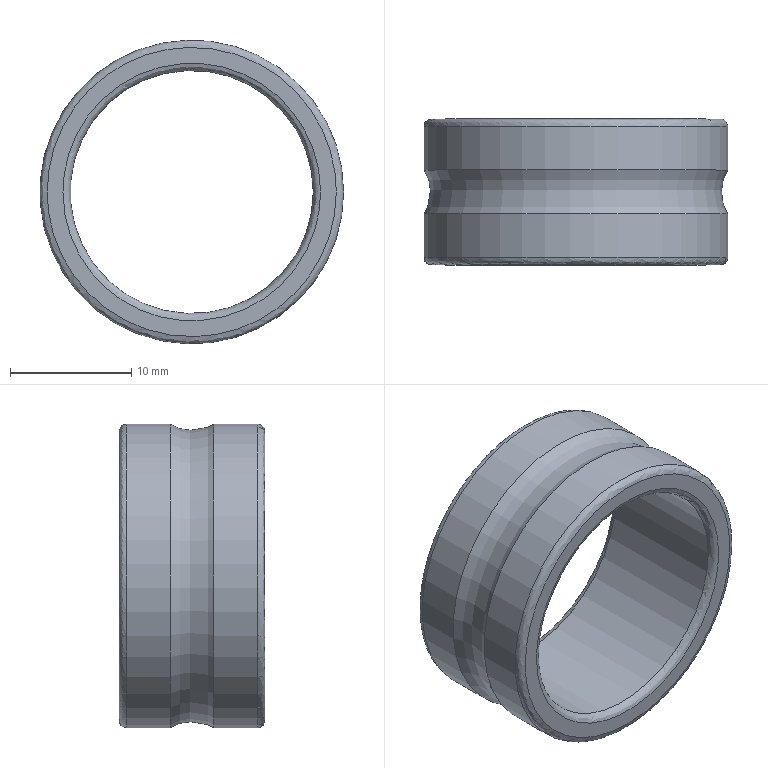Part | STEP file | BF-20_id1366_x_t | 1 solid | 10 faces | box 25 x 12 x 25 mm | volume 2005 mm3 | other 5 | cylinder 3 | plane 2 | commonest cylinder face diameters 25 x2 20 x1
STEP:
#1=CARTESIAN_POINT('',(0.,0.,0.));
#2=DIRECTION('',(0.,0.,1.));
#3=DIRECTION('',(1.,0.,0.));
#4=AXIS2_PLACEMENT_3D('',#1,#2,#3);
#5=CARTESIAN_POINT('',(-256.,-73.867,-165.5));
#6=VERTEX_POINT('',#5);
#7=CARTESIAN_POINT('',(-268.5,-73.867,-165.5));
#8=DIRECTION('',(0.,-1.,0.));
#9=DIRECTION('',(1.,0.,0.));
#10=AXIS2_PLACEMENT_3D('',#7,#8,#9);
#11=CIRCLE('',#10,12.5);
#12=CARTESIAN_POINT('',(-253.,-72.064,-165.5));
#13=DIRECTION('',(0.,0.,1.));
#14=DIRECTION('',(1.,0.,0.));
#15=AXIS2_PLACEMENT_3D('',#12,#13,#14);
#16=CIRCLE('',#15,3.5);
#17=CARTESIAN_POINT('',(-268.5,-72.064,-165.5));
#18=DIRECTION('',(0.,-1.,0.));
#19=AXIS1_PLACEMENT('',#17,#18);
#20=SURFACE_OF_REVOLUTION('',#16,#19);
#21=CARTESIAN_POINT('',(0.,3.683));
#22=DIRECTION('',(1.,0.));
#23=VECTOR('',#22,1.);
#24=LINE('',#21,#23);
#25=(GEOMETRIC_REPRESENTATION_CONTEXT(2)PARAMETRIC_REPRESENTATION_CONTEXT()REPRESENTATION_CONTEXT('',''));
#26=DEFINITIONAL_REPRESENTATION('',(#24),#25);
#27=PCURVE('',#20,#26);
#28=CARTESIAN_POINT('',(-268.5,-80.904,-165.5));
#29=DIRECTION('',(0.,-1.,0.));
#30=DIRECTION('',(1.,0.,0.));
#31=AXIS2_PLACEMENT_3D('',#28,#29,#30);
#32=CYLINDRICAL_SURFACE('',#31,12.5);
#33=CARTESIAN_POINT('',(0.,-7.037));
#34=DIRECTION('',(1.,0.));
#35=VECTOR('',#34,1.);
#36=LINE('',#33,#35);
#37=(GEOMETRIC_REPRESENTATION_CONTEXT(2)PARAMETRIC_REPRESENTATION_CONTEXT()REPRESENTATION_CONTEXT('',''));
#38=DEFINITIONAL_REPRESENTATION('',(#36),#37);
#39=PCURVE('',#32,#38);
#40=SURFACE_CURVE('',#11,(#27,#39),.PCURVE_S1.);
#41=EDGE_CURVE('',#6,#6,#40,.T.);
#42=ORIENTED_EDGE('',*,*,#41,.F.);
#43=CARTESIAN_POINT('',(-256.,-70.262,-165.5));
#44=VERTEX_POINT('',#43);
#45=CARTESIAN_POINT('',(-256.,-70.262,-165.5));
#46=CARTESIAN_POINT('',(-256.328,-70.808,-165.5));
#47=CARTESIAN_POINT('',(-256.534,-71.419,-165.5));
#48=CARTESIAN_POINT('',(-256.604,-72.064,-165.5));
#49=CARTESIAN_POINT('',(-256.534,-72.709,-165.5));
#50=CARTESIAN_POINT('',(-256.328,-73.321,-165.5));
#51=CARTESIAN_POINT('',(-256.,-73.867,-165.5));
#52=(BOUNDED_CURVE()B_SPLINE_CURVE(6,(#45,#46,#47,#48,#49,#50,#51),.UNSPECIFIED.,.F.,.F.)B_SPLINE_CURVE_WITH_KNOTS((7,7),(2.6,3.683),.PIECEWISE_BEZIER_KNOTS.)CURVE()GEOMETRIC_REPRESENTATION_ITEM()RATIONAL_B_SPLINE_CURVE((1.015,1.005,0.999,0.9971,0.999,1.005,1.015))REPRESENTATION_ITEM(''));
#53=CARTESIAN_POINT('',(0.,0.));
#54=DIRECTION('',(0.,1.));
#55=VECTOR('',#54,1.);
#56=LINE('',#53,#55);
#57=(GEOMETRIC_REPRESENTATION_CONTEXT(2)PARAMETRIC_REPRESENTATION_CONTEXT()REPRESENTATION_CONTEXT('',''));
#58=DEFINITIONAL_REPRESENTATION('',(#56),#57);
#59=PCURVE('',#20,#58);
#60=CARTESIAN_POINT('',(6.283,0.));
#61=DIRECTION('',(0.,1.));
#62=VECTOR('',#61,1.);
#63=LINE('',#60,#62);
#64=(GEOMETRIC_REPRESENTATION_CONTEXT(2)PARAMETRIC_REPRESENTATION_CONTEXT()REPRESENTATION_CONTEXT('',''));
#65=DEFINITIONAL_REPRESENTATION('',(#63),#64);
#66=PCURVE('',#20,#65);
#67=SEAM_CURVE('',#52,(#59,#66),.PCURVE_S1.);
#68=EDGE_CURVE('',#44,#6,#67,.T.);
#69=ORIENTED_EDGE('',*,*,#68,.F.);
#70=CARTESIAN_POINT('',(-268.5,-70.262,-165.5));
#71=DIRECTION('',(0.,1.,0.));
#72=DIRECTION('',(1.,0.,0.));
#73=AXIS2_PLACEMENT_3D('',#70,#71,#72);
#74=CIRCLE('',#73,12.5);
#75=CARTESIAN_POINT('',(6.283,2.6));
#76=DIRECTION('',(-1.,0.));
#77=VECTOR('',#76,1.);
#78=LINE('',#75,#77);
#79=(GEOMETRIC_REPRESENTATION_CONTEXT(2)PARAMETRIC_REPRESENTATION_CONTEXT()REPRESENTATION_CONTEXT('',''));
#80=DEFINITIONAL_REPRESENTATION('',(#78),#79);
#81=PCURVE('',#20,#80);
#82=CARTESIAN_POINT('',(-268.5,-80.904,-165.5));
#83=DIRECTION('',(0.,-1.,0.));
#84=DIRECTION('',(1.,0.,0.));
#85=AXIS2_PLACEMENT_3D('',#82,#83,#84);
#86=CYLINDRICAL_SURFACE('',#85,12.5);
#87=CARTESIAN_POINT('',(6.283,-10.642));
#88=DIRECTION('',(-1.,0.));
#89=VECTOR('',#88,1.);
#90=LINE('',#87,#89);
#91=(GEOMETRIC_REPRESENTATION_CONTEXT(2)PARAMETRIC_REPRESENTATION_CONTEXT()REPRESENTATION_CONTEXT('',''));
#92=DEFINITIONAL_REPRESENTATION('',(#90),#91);
#93=PCURVE('',#86,#92);
#94=SURFACE_CURVE('',#74,(#81,#93),.PCURVE_S1.);
#95=EDGE_CURVE('',#44,#44,#94,.T.);
#96=ORIENTED_EDGE('',*,*,#95,.F.);
#97=ORIENTED_EDGE('',*,*,#68,.T.);
#98=EDGE_LOOP('',(#42,#69,#96,#97));
#99=FACE_BOUND('',#98,.T.);
#100=ADVANCED_FACE('',(#99),#20,.T.);
#101=CARTESIAN_POINT('',(-256.,-77.464,-165.5));
#102=VERTEX_POINT('',#101);
#103=CARTESIAN_POINT('',(-268.5,-77.464,-165.5));
#104=DIRECTION('',(0.,-1.,0.));
#105=DIRECTION('',(1.,0.,0.));
#106=AXIS2_PLACEMENT_3D('',#103,#104,#105);
#107=CIRCLE('',#106,12.5);
#108=CARTESIAN_POINT('',(0.,-3.439));
#109=DIRECTION('',(1.,0.));
#110=VECTOR('',#109,1.);
#111=LINE('',#108,#110);
#112=(GEOMETRIC_REPRESENTATION_CONTEXT(2)PARAMETRIC_REPRESENTATION_CONTEXT()REPRESENTATION_CONTEXT('',''));
#113=DEFINITIONAL_REPRESENTATION('',(#111),#112);
#114=PCURVE('',#32,#113);
#115=CARTESIAN_POINT('',(-256.6,-77.464,-165.5));
#116=DIRECTION('',(0.,0.,1.));
#117=DIRECTION('',(1.,0.,0.));
#118=AXIS2_PLACEMENT_3D('',#115,#116,#117);
#119=CIRCLE('',#118,0.6);
#120=CARTESIAN_POINT('',(-268.5,-77.464,-165.5));
#121=DIRECTION('',(0.,-1.,0.));
#122=AXIS1_PLACEMENT('',#120,#121);
#123=SURFACE_OF_REVOLUTION('',#119,#122);
#124=CARTESIAN_POINT('',(0.,6.283));
#125=DIRECTION('',(1.,0.));
#126=VECTOR('',#125,1.);
#127=LINE('',#124,#126);
#128=(GEOMETRIC_REPRESENTATION_CONTEXT(2)PARAMETRIC_REPRESENTATION_CONTEXT()REPRESENTATION_CONTEXT('',''));
#129=DEFINITIONAL_REPRESENTATION('',(#127),#128);
#130=PCURVE('',#123,#129);
#131=SURFACE_CURVE('',#107,(#114,#130),.PCURVE_S1.);
#132=EDGE_CURVE('',#102,#102,#131,.T.);
#133=ORIENTED_EDGE('',*,*,#132,.F.);
#134=CARTESIAN_POINT('',(-256.,-73.867,-165.5));
#135=CARTESIAN_POINT('',(-256.,-77.464,-165.5));
#136=B_SPLINE_CURVE_WITH_KNOTS('',1,(#134,#135),.UNSPECIFIED.,.F.,.F.,(2,2),(-7.037,-3.439),.PIECEWISE_BEZIER_KNOTS.);
#137=CARTESIAN_POINT('',(0.,0.));
#138=DIRECTION('',(0.,1.));
#139=VECTOR('',#138,1.);
#140=LINE('',#137,#139);
#141=(GEOMETRIC_REPRESENTATION_CONTEXT(2)PARAMETRIC_REPRESENTATION_CONTEXT()REPRESENTATION_CONTEXT('',''));
#142=DEFINITIONAL_REPRESENTATION('',(#140),#141);
#143=PCURVE('',#32,#142);
#144=CARTESIAN_POINT('',(6.283,0.));
#145=DIRECTION('',(0.,1.));
#146=VECTOR('',#145,1.);
#147=LINE('',#144,#146);
#148=(GEOMETRIC_REPRESENTATION_CONTEXT(2)PARAMETRIC_REPRESENTATION_CONTEXT()REPRESENTATION_CONTEXT('',''));
#149=DEFINITIONAL_REPRESENTATION('',(#147),#148);
#150=PCURVE('',#32,#149);
#151=SEAM_CURVE('',#136,(#143,#150),.PCURVE_S1.);
#152=EDGE_CURVE('',#6,#102,#151,.T.);
#153=ORIENTED_EDGE('',*,*,#152,.F.);
#154=ORIENTED_EDGE('',*,*,#41,.T.);
#155=ORIENTED_EDGE('',*,*,#152,.T.);
#156=EDGE_LOOP('',(#133,#153,#154,#155));
#157=FACE_BOUND('',#156,.T.);
#158=ADVANCED_FACE('',(#157),#32,.T.);
#159=ORIENTED_EDGE('',*,*,#95,.T.);
#160=CARTESIAN_POINT('',(-256.,-66.664,-165.5));
#161=VERTEX_POINT('',#160);
#162=CARTESIAN_POINT('',(-256.,-66.664,-165.5));
#163=CARTESIAN_POINT('',(-256.,-70.262,-165.5));
#164=B_SPLINE_CURVE_WITH_KNOTS('',1,(#162,#163),.UNSPECIFIED.,.F.,.F.,(2,2),(-14.239,-10.642),.PIECEWISE_BEZIER_KNOTS.);
#165=CARTESIAN_POINT('',(0.,0.));
#166=DIRECTION('',(0.,1.));
#167=VECTOR('',#166,1.);
#168=LINE('',#165,#167);
#169=(GEOMETRIC_REPRESENTATION_CONTEXT(2)PARAMETRIC_REPRESENTATION_CONTEXT()REPRESENTATION_CONTEXT('',''));
#170=DEFINITIONAL_REPRESENTATION('',(#168),#169);
#171=PCURVE('',#86,#170);
#172=CARTESIAN_POINT('',(6.283,0.));
#173=DIRECTION('',(0.,1.));
#174=VECTOR('',#173,1.);
#175=LINE('',#172,#174);
#176=(GEOMETRIC_REPRESENTATION_CONTEXT(2)PARAMETRIC_REPRESENTATION_CONTEXT()REPRESENTATION_CONTEXT('',''));
#177=DEFINITIONAL_REPRESENTATION('',(#175),#176);
#178=PCURVE('',#86,#177);
#179=SEAM_CURVE('',#164,(#171,#178),.PCURVE_S1.);
#180=EDGE_CURVE('',#161,#44,#179,.T.);
#181=ORIENTED_EDGE('',*,*,#180,.F.);
#182=CARTESIAN_POINT('',(-268.5,-66.664,-165.5));
#183=DIRECTION('',(0.,1.,0.));
#184=DIRECTION('',(1.,0.,0.));
#185=AXIS2_PLACEMENT_3D('',#182,#183,#184);
#186=CIRCLE('',#185,12.5);
#187=CARTESIAN_POINT('',(6.283,-14.239));
#188=DIRECTION('',(-1.,0.));
#189=VECTOR('',#188,1.);
#190=LINE('',#187,#189);
#191=(GEOMETRIC_REPRESENTATION_CONTEXT(2)PARAMETRIC_REPRESENTATION_CONTEXT()REPRESENTATION_CONTEXT('',''));
#192=DEFINITIONAL_REPRESENTATION('',(#190),#191);
#193=PCURVE('',#86,#192);
#194=CARTESIAN_POINT('',(-256.6,-66.664,-165.5));
#195=DIRECTION('',(0.,0.,1.));
#196=DIRECTION('',(1.,0.,0.));
#197=AXIS2_PLACEMENT_3D('',#194,#195,#196);
#198=CIRCLE('',#197,0.6);
#199=CARTESIAN_POINT('',(-268.5,-66.664,-165.5));
#200=DIRECTION('',(0.,-1.,0.));
#201=AXIS1_PLACEMENT('',#199,#200);
#202=SURFACE_OF_REVOLUTION('',#198,#201);
#203=CARTESIAN_POINT('',(6.283,6.283));
#204=DIRECTION('',(-1.,0.));
#205=VECTOR('',#204,1.);
#206=LINE('',#203,#205);
#207=(GEOMETRIC_REPRESENTATION_CONTEXT(2)PARAMETRIC_REPRESENTATION_CONTEXT()REPRESENTATION_CONTEXT('',''));
#208=DEFINITIONAL_REPRESENTATION('',(#206),#207);
#209=PCURVE('',#202,#208);
#210=SURFACE_CURVE('',#186,(#193,#209),.PCURVE_S1.);
#211=EDGE_CURVE('',#161,#161,#210,.T.);
#212=ORIENTED_EDGE('',*,*,#211,.F.);
#213=ORIENTED_EDGE('',*,*,#180,.T.);
#214=EDGE_LOOP('',(#159,#181,#212,#213));
#215=FACE_BOUND('',#214,.T.);
#216=ADVANCED_FACE('',(#215),#86,.T.);
#217=CARTESIAN_POINT('',(-280.4,-78.064,-165.5));
#218=VERTEX_POINT('',#217);
#219=CARTESIAN_POINT('',(-256.6,-78.064,-165.5));
#220=VERTEX_POINT('',#219);
#221=CARTESIAN_POINT('',(-280.4,-78.064,-165.5));
#222=CARTESIAN_POINT('',(-280.4,-78.064,-141.7));
#223=CARTESIAN_POINT('',(-256.6,-78.064,-141.7));
#224=CARTESIAN_POINT('',(-256.6,-78.064,-165.5));
#225=(BOUNDED_CURVE()B_SPLINE_CURVE(3,(#221,#222,#223,#224),.UNSPECIFIED.,.F.,.F.)B_SPLINE_CURVE_WITH_KNOTS((4,4),(0.,1.),.PIECEWISE_BEZIER_KNOTS.)CURVE()GEOMETRIC_REPRESENTATION_ITEM()RATIONAL_B_SPLINE_CURVE((1.,0.3333,0.3333,1.))REPRESENTATION_ITEM(''));
#226=CARTESIAN_POINT('',(3.142,4.712));
#227=CARTESIAN_POINT('',(3.111,4.712));
#228=CARTESIAN_POINT('',(3.048,4.712));
#229=CARTESIAN_POINT('',(2.944,4.712));
#230=CARTESIAN_POINT('',(2.83,4.712));
#231=CARTESIAN_POINT('',(2.706,4.712));
#232=CARTESIAN_POINT('',(2.571,4.712));
#233=CARTESIAN_POINT('',(2.426,4.712));
#234=CARTESIAN_POINT('',(2.27,4.712));
#235=CARTESIAN_POINT('',(2.105,4.712));
#236=CARTESIAN_POINT('',(1.931,4.712));
#237=CARTESIAN_POINT('',(1.753,4.712));
#238=CARTESIAN_POINT('',(1.571,4.712));
#239=CARTESIAN_POINT('',(1.389,4.712));
#240=CARTESIAN_POINT('',(1.21,4.712));
#241=CARTESIAN_POINT('',(1.037,4.712));
#242=CARTESIAN_POINT('',(0.8717,4.712));
#243=CARTESIAN_POINT('',(0.7158,4.712));
#244=CARTESIAN_POINT('',(0.5703,4.712));
#245=CARTESIAN_POINT('',(0.4356,4.712));
#246=CARTESIAN_POINT('',(0.3115,4.712));
#247=CARTESIAN_POINT('',(0.1977,4.712));
#248=CARTESIAN_POINT('',(0.09367,4.712));
#249=CARTESIAN_POINT('',(0.0303,4.712));
#250=CARTESIAN_POINT('',(0.,4.712));
#251=B_SPLINE_CURVE_WITH_KNOTS('',3,(#226,#227,#228,#229,#230,#231,#232,#233,#234,#235,#236,#237,#238,#239,#240,#241,#242,#243,#244,#245,#246,#247,#248,#249,#250),.UNSPECIFIED.,.F.,.F.,(4,1,1,1,1,1,1,1,1,1,1,1,1,1,1,1,1,1,1,1,1,1,4),(0.,0.04545,0.09091,0.1364,0.1818,0.2273,0.2727,0.3182,0.3636,0.4091,0.4545,0.5,0.5455,0.5909,0.6364,0.6818,0.7273,0.7727,0.8182,0.8636,0.9091,0.9545,1.),.QUASI_UNIFORM_KNOTS.);
#252=(GEOMETRIC_REPRESENTATION_CONTEXT(2)PARAMETRIC_REPRESENTATION_CONTEXT()REPRESENTATION_CONTEXT('',''));
#253=DEFINITIONAL_REPRESENTATION('',(#251),#252);
#254=PCURVE('',#123,#253);
#255=CARTESIAN_POINT('',(-268.5,-78.064,-154.9));
#256=DIRECTION('',(0.,1.,0.));
#257=DIRECTION('',(-1.,0.,0.));
#258=AXIS2_PLACEMENT_3D('',#255,#256,#257);
#259=PLANE('',#258);
#260=CARTESIAN_POINT('',(11.9,-10.6));
#261=CARTESIAN_POINT('',(11.9,13.2));
#262=CARTESIAN_POINT('',(-11.9,13.2));
#263=CARTESIAN_POINT('',(-11.9,-10.6));
#264=(BOUNDED_CURVE()B_SPLINE_CURVE(3,(#260,#261,#262,#263),.UNSPECIFIED.,.F.,.F.)B_SPLINE_CURVE_WITH_KNOTS((4,4),(0.,1.),.PIECEWISE_BEZIER_KNOTS.)CURVE()GEOMETRIC_REPRESENTATION_ITEM()RATIONAL_B_SPLINE_CURVE((1.,0.3333,0.3333,1.))REPRESENTATION_ITEM(''));
#265=(GEOMETRIC_REPRESENTATION_CONTEXT(2)PARAMETRIC_REPRESENTATION_CONTEXT()REPRESENTATION_CONTEXT('',''));
#266=DEFINITIONAL_REPRESENTATION('',(#264),#265);
#267=PCURVE('',#259,#266);
#268=SURFACE_CURVE('',#225,(#254,#267),.PCURVE_S1.);
#269=EDGE_CURVE('',#218,#220,#268,.T.);
#270=ORIENTED_EDGE('',*,*,#269,.F.);
#271=CARTESIAN_POINT('',(-256.6,-78.064,-165.5));
#272=CARTESIAN_POINT('',(-256.6,-78.064,-189.3));
#273=CARTESIAN_POINT('',(-280.4,-78.064,-189.3));
#274=CARTESIAN_POINT('',(-280.4,-78.064,-165.5));
#275=(BOUNDED_CURVE()B_SPLINE_CURVE(3,(#271,#272,#273,#274),.UNSPECIFIED.,.F.,.F.)B_SPLINE_CURVE_WITH_KNOTS((4,4),(0.,1.),.PIECEWISE_BEZIER_KNOTS.)CURVE()GEOMETRIC_REPRESENTATION_ITEM()RATIONAL_B_SPLINE_CURVE((1.,0.3333,0.3333,1.))REPRESENTATION_ITEM(''));
#276=CARTESIAN_POINT('',(6.283,4.712));
#277=CARTESIAN_POINT('',(6.253,4.712));
#278=CARTESIAN_POINT('',(6.19,4.712));
#279=CARTESIAN_POINT('',(6.085,4.712));
#280=CARTESIAN_POINT('',(5.972,4.712));
#281=CARTESIAN_POINT('',(5.848,4.712));
#282=CARTESIAN_POINT('',(5.713,4.712));
#283=CARTESIAN_POINT('',(5.567,4.712));
#284=CARTESIAN_POINT('',(5.412,4.712));
#285=CARTESIAN_POINT('',(5.246,4.712));
#286=CARTESIAN_POINT('',(5.073,4.712));
#287=CARTESIAN_POINT('',(4.894,4.712));
#288=CARTESIAN_POINT('',(4.712,4.712));
#289=CARTESIAN_POINT('',(4.531,4.712));
#290=CARTESIAN_POINT('',(4.352,4.712));
#291=CARTESIAN_POINT('',(4.179,4.712));
#292=CARTESIAN_POINT('',(4.013,4.712));
#293=CARTESIAN_POINT('',(3.857,4.712));
#294=CARTESIAN_POINT('',(3.712,4.712));
#295=CARTESIAN_POINT('',(3.577,4.712));
#296=CARTESIAN_POINT('',(3.453,4.712));
#297=CARTESIAN_POINT('',(3.339,4.712));
#298=CARTESIAN_POINT('',(3.235,4.712));
#299=CARTESIAN_POINT('',(3.172,4.712));
#300=CARTESIAN_POINT('',(3.142,4.712));
#301=B_SPLINE_CURVE_WITH_KNOTS('',3,(#276,#277,#278,#279,#280,#281,#282,#283,#284,#285,#286,#287,#288,#289,#290,#291,#292,#293,#294,#295,#296,#297,#298,#299,#300),.UNSPECIFIED.,.F.,.F.,(4,1,1,1,1,1,1,1,1,1,1,1,1,1,1,1,1,1,1,1,1,1,4),(0.,0.04545,0.09091,0.1364,0.1818,0.2273,0.2727,0.3182,0.3636,0.4091,0.4545,0.5,0.5455,0.5909,0.6364,0.6818,0.7273,0.7727,0.8182,0.8636,0.9091,0.9545,1.),.QUASI_UNIFORM_KNOTS.);
#302=(GEOMETRIC_REPRESENTATION_CONTEXT(2)PARAMETRIC_REPRESENTATION_CONTEXT()REPRESENTATION_CONTEXT('',''));
#303=DEFINITIONAL_REPRESENTATION('',(#301),#302);
#304=PCURVE('',#123,#303);
#305=CARTESIAN_POINT('',(-11.9,-10.6));
#306=CARTESIAN_POINT('',(-11.9,-34.4));
#307=CARTESIAN_POINT('',(11.9,-34.4));
#308=CARTESIAN_POINT('',(11.9,-10.6));
#309=(BOUNDED_CURVE()B_SPLINE_CURVE(3,(#305,#306,#307,#308),.UNSPECIFIED.,.F.,.F.)B_SPLINE_CURVE_WITH_KNOTS((4,4),(0.,1.),.PIECEWISE_BEZIER_KNOTS.)CURVE()GEOMETRIC_REPRESENTATION_ITEM()RATIONAL_B_SPLINE_CURVE((1.,0.3333,0.3333,1.))REPRESENTATION_ITEM(''));
#310=(GEOMETRIC_REPRESENTATION_CONTEXT(2)PARAMETRIC_REPRESENTATION_CONTEXT()REPRESENTATION_CONTEXT('',''));
#311=DEFINITIONAL_REPRESENTATION('',(#309),#310);
#312=PCURVE('',#259,#311);
#313=SURFACE_CURVE('',#275,(#304,#312),.PCURVE_S1.);
#314=EDGE_CURVE('',#220,#218,#313,.T.);
#315=ORIENTED_EDGE('',*,*,#314,.F.);
#316=CARTESIAN_POINT('',(-256.6,-78.064,-165.5));
#317=CARTESIAN_POINT('',(-256.44,-78.064,-165.5));
#318=CARTESIAN_POINT('',(-256.283,-78.013,-165.5));
#319=CARTESIAN_POINT('',(-256.149,-77.916,-165.5));
#320=CARTESIAN_POINT('',(-256.051,-77.781,-165.5));
#321=CARTESIAN_POINT('',(-256.,-77.625,-165.5));
#322=CARTESIAN_POINT('',(-256.,-77.464,-165.5));
#323=(BOUNDED_CURVE()B_SPLINE_CURVE(6,(#316,#317,#318,#319,#320,#321,#322),.UNSPECIFIED.,.F.,.F.)B_SPLINE_CURVE_WITH_KNOTS((7,7),(4.712,6.283),.PIECEWISE_BEZIER_KNOTS.)CURVE()GEOMETRIC_REPRESENTATION_ITEM()RATIONAL_B_SPLINE_CURVE((1.031,1.01,0.9979,0.994,0.9979,1.01,1.031))REPRESENTATION_ITEM(''));
#324=CARTESIAN_POINT('',(6.283,0.));
#325=DIRECTION('',(0.,1.));
#326=VECTOR('',#325,1.);
#327=LINE('',#324,#326);
#328=(GEOMETRIC_REPRESENTATION_CONTEXT(2)PARAMETRIC_REPRESENTATION_CONTEXT()REPRESENTATION_CONTEXT('',''));
#329=DEFINITIONAL_REPRESENTATION('',(#327),#328);
#330=PCURVE('',#123,#329);
#331=CARTESIAN_POINT('',(0.,0.));
#332=DIRECTION('',(0.,1.));
#333=VECTOR('',#332,1.);
#334=LINE('',#331,#333);
#335=(GEOMETRIC_REPRESENTATION_CONTEXT(2)PARAMETRIC_REPRESENTATION_CONTEXT()REPRESENTATION_CONTEXT('',''));
#336=DEFINITIONAL_REPRESENTATION('',(#334),#335);
#337=PCURVE('',#123,#336);
#338=SEAM_CURVE('',#323,(#330,#337),.PCURVE_S1.);
#339=EDGE_CURVE('',#220,#102,#338,.T.);
#340=ORIENTED_EDGE('',*,*,#339,.T.);
#341=ORIENTED_EDGE('',*,*,#132,.F.);
#342=ORIENTED_EDGE('',*,*,#339,.F.);
#343=EDGE_LOOP('',(#270,#315,#340,#341,#342));
#344=FACE_BOUND('',#343,.F.);
#345=ADVANCED_FACE('',(#344),#123,.F.);
#346=ORIENTED_EDGE('',*,*,#211,.F.);
#347=CARTESIAN_POINT('',(-256.6,-66.064,-165.5));
#348=VERTEX_POINT('',#347);
#349=CARTESIAN_POINT('',(-256.,-66.664,-165.5));
#350=CARTESIAN_POINT('',(-256.,-66.504,-165.5));
#351=CARTESIAN_POINT('',(-256.051,-66.348,-165.5));
#352=CARTESIAN_POINT('',(-256.149,-66.213,-165.5));
#353=CARTESIAN_POINT('',(-256.283,-66.115,-165.5));
#354=CARTESIAN_POINT('',(-256.44,-66.064,-165.5));
#355=CARTESIAN_POINT('',(-256.6,-66.064,-165.5));
#356=(BOUNDED_CURVE()B_SPLINE_CURVE(6,(#349,#350,#351,#352,#353,#354,#355),.UNSPECIFIED.,.F.,.F.)B_SPLINE_CURVE_WITH_KNOTS((7,7),(0.,1.571),.PIECEWISE_BEZIER_KNOTS.)CURVE()GEOMETRIC_REPRESENTATION_ITEM()RATIONAL_B_SPLINE_CURVE((1.031,1.01,0.9979,0.994,0.9979,1.01,1.031))REPRESENTATION_ITEM(''));
#357=CARTESIAN_POINT('',(6.283,6.283));
#358=DIRECTION('',(0.,1.));
#359=VECTOR('',#358,1.);
#360=LINE('',#357,#359);
#361=(GEOMETRIC_REPRESENTATION_CONTEXT(2)PARAMETRIC_REPRESENTATION_CONTEXT()REPRESENTATION_CONTEXT('',''));
#362=DEFINITIONAL_REPRESENTATION('',(#360),#361);
#363=PCURVE('',#202,#362);
#364=CARTESIAN_POINT('',(0.,6.283));
#365=DIRECTION('',(0.,1.));
#366=VECTOR('',#365,1.);
#367=LINE('',#364,#366);
#368=(GEOMETRIC_REPRESENTATION_CONTEXT(2)PARAMETRIC_REPRESENTATION_CONTEXT()REPRESENTATION_CONTEXT('',''));
#369=DEFINITIONAL_REPRESENTATION('',(#367),#368);
#370=PCURVE('',#202,#369);
#371=SEAM_CURVE('',#356,(#363,#370),.PCURVE_S1.);
#372=EDGE_CURVE('',#161,#348,#371,.T.);
#373=ORIENTED_EDGE('',*,*,#372,.T.);
#374=CARTESIAN_POINT('',(-280.4,-66.064,-165.5));
#375=VERTEX_POINT('',#374);
#376=CARTESIAN_POINT('',(-280.4,-66.064,-165.5));
#377=CARTESIAN_POINT('',(-280.4,-66.064,-189.3));
#378=CARTESIAN_POINT('',(-256.6,-66.064,-189.3));
#379=CARTESIAN_POINT('',(-256.6,-66.064,-165.5));
#380=(BOUNDED_CURVE()B_SPLINE_CURVE(3,(#376,#377,#378,#379),.UNSPECIFIED.,.F.,.F.)B_SPLINE_CURVE_WITH_KNOTS((4,4),(0.,1.),.PIECEWISE_BEZIER_KNOTS.)CURVE()GEOMETRIC_REPRESENTATION_ITEM()RATIONAL_B_SPLINE_CURVE((1.,0.3333,0.3333,1.))REPRESENTATION_ITEM(''));
#381=CARTESIAN_POINT('',(3.142,7.854));
#382=CARTESIAN_POINT('',(3.172,7.854));
#383=CARTESIAN_POINT('',(3.235,7.854));
#384=CARTESIAN_POINT('',(3.339,7.854));
#385=CARTESIAN_POINT('',(3.453,7.854));
#386=CARTESIAN_POINT('',(3.577,7.854));
#387=CARTESIAN_POINT('',(3.712,7.854));
#388=CARTESIAN_POINT('',(3.857,7.854));
#389=CARTESIAN_POINT('',(4.013,7.854));
#390=CARTESIAN_POINT('',(4.179,7.854));
#391=CARTESIAN_POINT('',(4.352,7.854));
#392=CARTESIAN_POINT('',(4.531,7.854));
#393=CARTESIAN_POINT('',(4.712,7.854));
#394=CARTESIAN_POINT('',(4.894,7.854));
#395=CARTESIAN_POINT('',(5.073,7.854));
#396=CARTESIAN_POINT('',(5.246,7.854));
#397=CARTESIAN_POINT('',(5.412,7.854));
#398=CARTESIAN_POINT('',(5.567,7.854));
#399=CARTESIAN_POINT('',(5.713,7.854));
#400=CARTESIAN_POINT('',(5.848,7.854));
#401=CARTESIAN_POINT('',(5.972,7.854));
#402=CARTESIAN_POINT('',(6.085,7.854));
#403=CARTESIAN_POINT('',(6.19,7.854));
#404=CARTESIAN_POINT('',(6.253,7.854));
#405=CARTESIAN_POINT('',(6.283,7.854));
#406=B_SPLINE_CURVE_WITH_KNOTS('',3,(#381,#382,#383,#384,#385,#386,#387,#388,#389,#390,#391,#392,#393,#394,#395,#396,#397,#398,#399,#400,#401,#402,#403,#404,#405),.UNSPECIFIED.,.F.,.F.,(4,1,1,1,1,1,1,1,1,1,1,1,1,1,1,1,1,1,1,1,1,1,4),(0.,0.04545,0.09091,0.1364,0.1818,0.2273,0.2727,0.3182,0.3636,0.4091,0.4545,0.5,0.5455,0.5909,0.6364,0.6818,0.7273,0.7727,0.8182,0.8636,0.9091,0.9545,1.),.QUASI_UNIFORM_KNOTS.);
#407=(GEOMETRIC_REPRESENTATION_CONTEXT(2)PARAMETRIC_REPRESENTATION_CONTEXT()REPRESENTATION_CONTEXT('',''));
#408=DEFINITIONAL_REPRESENTATION('',(#406),#407);
#409=PCURVE('',#202,#408);
#410=CARTESIAN_POINT('',(-268.5,-66.064,-154.9));
#411=DIRECTION('',(0.,-1.,0.));
#412=DIRECTION('',(1.,0.,0.));
#413=AXIS2_PLACEMENT_3D('',#410,#411,#412);
#414=PLANE('',#413);
#415=CARTESIAN_POINT('',(-11.9,-10.6));
#416=CARTESIAN_POINT('',(-11.9,-34.4));
#417=CARTESIAN_POINT('',(11.9,-34.4));
#418=CARTESIAN_POINT('',(11.9,-10.6));
#419=(BOUNDED_CURVE()B_SPLINE_CURVE(3,(#415,#416,#417,#418),.UNSPECIFIED.,.F.,.F.)B_SPLINE_CURVE_WITH_KNOTS((4,4),(0.,1.),.PIECEWISE_BEZIER_KNOTS.)CURVE()GEOMETRIC_REPRESENTATION_ITEM()RATIONAL_B_SPLINE_CURVE((1.,0.3333,0.3333,1.))REPRESENTATION_ITEM(''));
#420=(GEOMETRIC_REPRESENTATION_CONTEXT(2)PARAMETRIC_REPRESENTATION_CONTEXT()REPRESENTATION_CONTEXT('',''));
#421=DEFINITIONAL_REPRESENTATION('',(#419),#420);
#422=PCURVE('',#414,#421);
#423=SURFACE_CURVE('',#380,(#409,#422),.PCURVE_S1.);
#424=EDGE_CURVE('',#375,#348,#423,.T.);
#425=ORIENTED_EDGE('',*,*,#424,.F.);
#426=CARTESIAN_POINT('',(-256.6,-66.064,-165.5));
#427=CARTESIAN_POINT('',(-256.6,-66.064,-141.7));
#428=CARTESIAN_POINT('',(-280.4,-66.064,-141.7));
#429=CARTESIAN_POINT('',(-280.4,-66.064,-165.5));
#430=(BOUNDED_CURVE()B_SPLINE_CURVE(3,(#426,#427,#428,#429),.UNSPECIFIED.,.F.,.F.)B_SPLINE_CURVE_WITH_KNOTS((4,4),(0.,1.),.PIECEWISE_BEZIER_KNOTS.)CURVE()GEOMETRIC_REPRESENTATION_ITEM()RATIONAL_B_SPLINE_CURVE((1.,0.3333,0.3333,1.))REPRESENTATION_ITEM(''));
#431=CARTESIAN_POINT('',(0.,7.854));
#432=CARTESIAN_POINT('',(0.0303,7.854));
#433=CARTESIAN_POINT('',(0.09367,7.854));
#434=CARTESIAN_POINT('',(0.1977,7.854));
#435=CARTESIAN_POINT('',(0.3115,7.854));
#436=CARTESIAN_POINT('',(0.4356,7.854));
#437=CARTESIAN_POINT('',(0.5703,7.854));
#438=CARTESIAN_POINT('',(0.7158,7.854));
#439=CARTESIAN_POINT('',(0.8717,7.854));
#440=CARTESIAN_POINT('',(1.037,7.854));
#441=CARTESIAN_POINT('',(1.21,7.854));
#442=CARTESIAN_POINT('',(1.389,7.854));
#443=CARTESIAN_POINT('',(1.571,7.854));
#444=CARTESIAN_POINT('',(1.753,7.854));
#445=CARTESIAN_POINT('',(1.931,7.854));
#446=CARTESIAN_POINT('',(2.105,7.854));
#447=CARTESIAN_POINT('',(2.27,7.854));
#448=CARTESIAN_POINT('',(2.426,7.854));
#449=CARTESIAN_POINT('',(2.571,7.854));
#450=CARTESIAN_POINT('',(2.706,7.854));
#451=CARTESIAN_POINT('',(2.83,7.854));
#452=CARTESIAN_POINT('',(2.944,7.854));
#453=CARTESIAN_POINT('',(3.048,7.854));
#454=CARTESIAN_POINT('',(3.111,7.854));
#455=CARTESIAN_POINT('',(3.142,7.854));
#456=B_SPLINE_CURVE_WITH_KNOTS('',3,(#431,#432,#433,#434,#435,#436,#437,#438,#439,#440,#441,#442,#443,#444,#445,#446,#447,#448,#449,#450,#451,#452,#453,#454,#455),.UNSPECIFIED.,.F.,.F.,(4,1,1,1,1,1,1,1,1,1,1,1,1,1,1,1,1,1,1,1,1,1,4),(0.,0.04545,0.09091,0.1364,0.1818,0.2273,0.2727,0.3182,0.3636,0.4091,0.4545,0.5,0.5455,0.5909,0.6364,0.6818,0.7273,0.7727,0.8182,0.8636,0.9091,0.9545,1.),.QUASI_UNIFORM_KNOTS.);
#457=(GEOMETRIC_REPRESENTATION_CONTEXT(2)PARAMETRIC_REPRESENTATION_CONTEXT()REPRESENTATION_CONTEXT('',''));
#458=DEFINITIONAL_REPRESENTATION('',(#456),#457);
#459=PCURVE('',#202,#458);
#460=CARTESIAN_POINT('',(11.9,-10.6));
#461=CARTESIAN_POINT('',(11.9,13.2));
#462=CARTESIAN_POINT('',(-11.9,13.2));
#463=CARTESIAN_POINT('',(-11.9,-10.6));
#464=(BOUNDED_CURVE()B_SPLINE_CURVE(3,(#460,#461,#462,#463),.UNSPECIFIED.,.F.,.F.)B_SPLINE_CURVE_WITH_KNOTS((4,4),(0.,1.),.PIECEWISE_BEZIER_KNOTS.)CURVE()GEOMETRIC_REPRESENTATION_ITEM()RATIONAL_B_SPLINE_CURVE((1.,0.3333,0.3333,1.))REPRESENTATION_ITEM(''));
#465=(GEOMETRIC_REPRESENTATION_CONTEXT(2)PARAMETRIC_REPRESENTATION_CONTEXT()REPRESENTATION_CONTEXT('',''));
#466=DEFINITIONAL_REPRESENTATION('',(#464),#465);
#467=PCURVE('',#414,#466);
#468=SURFACE_CURVE('',#430,(#459,#467),.PCURVE_S1.);
#469=EDGE_CURVE('',#348,#375,#468,.T.);
#470=ORIENTED_EDGE('',*,*,#469,.F.);
#471=ORIENTED_EDGE('',*,*,#372,.F.);
#472=EDGE_LOOP('',(#346,#373,#425,#470,#471));
#473=FACE_BOUND('',#472,.F.);
#474=ADVANCED_FACE('',(#473),#202,.F.);
#475=ORIENTED_EDGE('',*,*,#314,.F.);
#476=ORIENTED_EDGE('',*,*,#269,.F.);
#477=EDGE_LOOP('',(#475,#476));
#478=FACE_BOUND('',#477,.T.);
#479=CARTESIAN_POINT('',(-279.1,-78.064,-165.5));
#480=VERTEX_POINT('',#479);
#481=CARTESIAN_POINT('',(-257.9,-78.064,-165.5));
#482=VERTEX_POINT('',#481);
#483=CARTESIAN_POINT('',(-279.1,-78.064,-165.5));
#484=CARTESIAN_POINT('',(-279.1,-78.064,-186.7));
#485=CARTESIAN_POINT('',(-257.9,-78.064,-186.7));
#486=CARTESIAN_POINT('',(-257.9,-78.064,-165.5));
#487=(BOUNDED_CURVE()B_SPLINE_CURVE(3,(#483,#484,#485,#486),.UNSPECIFIED.,.F.,.F.)B_SPLINE_CURVE_WITH_KNOTS((4,4),(0.,1.),.PIECEWISE_BEZIER_KNOTS.)CURVE()GEOMETRIC_REPRESENTATION_ITEM()RATIONAL_B_SPLINE_CURVE((1.,0.3333,0.3333,1.))REPRESENTATION_ITEM(''));
#488=CARTESIAN_POINT('',(10.6,-10.6));
#489=CARTESIAN_POINT('',(10.6,-31.8));
#490=CARTESIAN_POINT('',(-10.6,-31.8));
#491=CARTESIAN_POINT('',(-10.6,-10.6));
#492=(BOUNDED_CURVE()B_SPLINE_CURVE(3,(#488,#489,#490,#491),.UNSPECIFIED.,.F.,.F.)B_SPLINE_CURVE_WITH_KNOTS((4,4),(0.,1.),.PIECEWISE_BEZIER_KNOTS.)CURVE()GEOMETRIC_REPRESENTATION_ITEM()RATIONAL_B_SPLINE_CURVE((1.,0.3333,0.3333,1.))REPRESENTATION_ITEM(''));
#493=(GEOMETRIC_REPRESENTATION_CONTEXT(2)PARAMETRIC_REPRESENTATION_CONTEXT()REPRESENTATION_CONTEXT('',''));
#494=DEFINITIONAL_REPRESENTATION('',(#492),#493);
#495=PCURVE('',#259,#494);
#496=CARTESIAN_POINT('',(-257.9,-77.464,-165.5));
#497=DIRECTION('',(0.,0.,1.));
#498=DIRECTION('',(1.,0.,0.));
#499=AXIS2_PLACEMENT_3D('',#496,#497,#498);
#500=CIRCLE('',#499,0.6);
#501=CARTESIAN_POINT('',(-268.5,-77.464,-165.5));
#502=DIRECTION('',(0.,-1.,0.));
#503=AXIS1_PLACEMENT('',#501,#502);
#504=SURFACE_OF_REVOLUTION('',#500,#503);
#505=CARTESIAN_POINT('',(3.142,4.712));
#506=CARTESIAN_POINT('',(3.172,4.712));
#507=CARTESIAN_POINT('',(3.235,4.712));
#508=CARTESIAN_POINT('',(3.339,4.712));
#509=CARTESIAN_POINT('',(3.453,4.712));
#510=CARTESIAN_POINT('',(3.577,4.712));
#511=CARTESIAN_POINT('',(3.712,4.712));
#512=CARTESIAN_POINT('',(3.857,4.712));
#513=CARTESIAN_POINT('',(4.013,4.712));
#514=CARTESIAN_POINT('',(4.179,4.712));
#515=CARTESIAN_POINT('',(4.352,4.712));
#516=CARTESIAN_POINT('',(4.531,4.712));
#517=CARTESIAN_POINT('',(4.712,4.712));
#518=CARTESIAN_POINT('',(4.894,4.712));
#519=CARTESIAN_POINT('',(5.073,4.712));
#520=CARTESIAN_POINT('',(5.246,4.712));
#521=CARTESIAN_POINT('',(5.412,4.712));
#522=CARTESIAN_POINT('',(5.567,4.712));
#523=CARTESIAN_POINT('',(5.713,4.712));
#524=CARTESIAN_POINT('',(5.848,4.712));
#525=CARTESIAN_POINT('',(5.972,4.712));
#526=CARTESIAN_POINT('',(6.085,4.712));
#527=CARTESIAN_POINT('',(6.19,4.712));
#528=CARTESIAN_POINT('',(6.253,4.712));
#529=CARTESIAN_POINT('',(6.283,4.712));
#530=B_SPLINE_CURVE_WITH_KNOTS('',3,(#505,#506,#507,#508,#509,#510,#511,#512,#513,#514,#515,#516,#517,#518,#519,#520,#521,#522,#523,#524,#525,#526,#527,#528,#529),.UNSPECIFIED.,.F.,.F.,(4,1,1,1,1,1,1,1,1,1,1,1,1,1,1,1,1,1,1,1,1,1,4),(0.,0.04545,0.09091,0.1364,0.1818,0.2273,0.2727,0.3182,0.3636,0.4091,0.4545,0.5,0.5455,0.5909,0.6364,0.6818,0.7273,0.7727,0.8182,0.8636,0.9091,0.9545,1.),.QUASI_UNIFORM_KNOTS.);
#531=(GEOMETRIC_REPRESENTATION_CONTEXT(2)PARAMETRIC_REPRESENTATION_CONTEXT()REPRESENTATION_CONTEXT('',''));
#532=DEFINITIONAL_REPRESENTATION('',(#530),#531);
#533=PCURVE('',#504,#532);
#534=SURFACE_CURVE('',#487,(#495,#533),.PCURVE_S1.);
#535=EDGE_CURVE('',#480,#482,#534,.T.);
#536=ORIENTED_EDGE('',*,*,#535,.F.);
#537=CARTESIAN_POINT('',(-257.9,-78.064,-165.5));
#538=CARTESIAN_POINT('',(-257.9,-78.064,-144.3));
#539=CARTESIAN_POINT('',(-279.1,-78.064,-144.3));
#540=CARTESIAN_POINT('',(-279.1,-78.064,-165.5));
#541=(BOUNDED_CURVE()B_SPLINE_CURVE(3,(#537,#538,#539,#540),.UNSPECIFIED.,.F.,.F.)B_SPLINE_CURVE_WITH_KNOTS((4,4),(0.,1.),.PIECEWISE_BEZIER_KNOTS.)CURVE()GEOMETRIC_REPRESENTATION_ITEM()RATIONAL_B_SPLINE_CURVE((1.,0.3333,0.3333,1.))REPRESENTATION_ITEM(''));
#542=CARTESIAN_POINT('',(-10.6,-10.6));
#543=CARTESIAN_POINT('',(-10.6,10.6));
#544=CARTESIAN_POINT('',(10.6,10.6));
#545=CARTESIAN_POINT('',(10.6,-10.6));
#546=(BOUNDED_CURVE()B_SPLINE_CURVE(3,(#542,#543,#544,#545),.UNSPECIFIED.,.F.,.F.)B_SPLINE_CURVE_WITH_KNOTS((4,4),(0.,1.),.PIECEWISE_BEZIER_KNOTS.)CURVE()GEOMETRIC_REPRESENTATION_ITEM()RATIONAL_B_SPLINE_CURVE((1.,0.3333,0.3333,1.))REPRESENTATION_ITEM(''));
#547=(GEOMETRIC_REPRESENTATION_CONTEXT(2)PARAMETRIC_REPRESENTATION_CONTEXT()REPRESENTATION_CONTEXT('',''));
#548=DEFINITIONAL_REPRESENTATION('',(#546),#547);
#549=PCURVE('',#259,#548);
#550=CARTESIAN_POINT('',(0.,4.712));
#551=CARTESIAN_POINT('',(0.0303,4.712));
#552=CARTESIAN_POINT('',(0.09367,4.712));
#553=CARTESIAN_POINT('',(0.1977,4.712));
#554=CARTESIAN_POINT('',(0.3115,4.712));
#555=CARTESIAN_POINT('',(0.4356,4.712));
#556=CARTESIAN_POINT('',(0.5703,4.712));
#557=CARTESIAN_POINT('',(0.7158,4.712));
#558=CARTESIAN_POINT('',(0.8717,4.712));
#559=CARTESIAN_POINT('',(1.037,4.712));
#560=CARTESIAN_POINT('',(1.21,4.712));
#561=CARTESIAN_POINT('',(1.389,4.712));
#562=CARTESIAN_POINT('',(1.571,4.712));
#563=CARTESIAN_POINT('',(1.753,4.712));
#564=CARTESIAN_POINT('',(1.931,4.712));
#565=CARTESIAN_POINT('',(2.105,4.712));
#566=CARTESIAN_POINT('',(2.27,4.712));
#567=CARTESIAN_POINT('',(2.426,4.712));
#568=CARTESIAN_POINT('',(2.571,4.712));
#569=CARTESIAN_POINT('',(2.706,4.712));
#570=CARTESIAN_POINT('',(2.83,4.712));
#571=CARTESIAN_POINT('',(2.944,4.712));
#572=CARTESIAN_POINT('',(3.048,4.712));
#573=CARTESIAN_POINT('',(3.111,4.712));
#574=CARTESIAN_POINT('',(3.142,4.712));
#575=B_SPLINE_CURVE_WITH_KNOTS('',3,(#550,#551,#552,#553,#554,#555,#556,#557,#558,#559,#560,#561,#562,#563,#564,#565,#566,#567,#568,#569,#570,#571,#572,#573,#574),.UNSPECIFIED.,.F.,.F.,(4,1,1,1,1,1,1,1,1,1,1,1,1,1,1,1,1,1,1,1,1,1,4),(0.,0.04545,0.09091,0.1364,0.1818,0.2273,0.2727,0.3182,0.3636,0.4091,0.4545,0.5,0.5455,0.5909,0.6364,0.6818,0.7273,0.7727,0.8182,0.8636,0.9091,0.9545,1.),.QUASI_UNIFORM_KNOTS.);
#576=(GEOMETRIC_REPRESENTATION_CONTEXT(2)PARAMETRIC_REPRESENTATION_CONTEXT()REPRESENTATION_CONTEXT('',''));
#577=DEFINITIONAL_REPRESENTATION('',(#575),#576);
#578=PCURVE('',#504,#577);
#579=SURFACE_CURVE('',#541,(#549,#578),.PCURVE_S1.);
#580=EDGE_CURVE('',#482,#480,#579,.T.);
#581=ORIENTED_EDGE('',*,*,#580,.F.);
#582=EDGE_LOOP('',(#536,#581));
#583=FACE_BOUND('',#582,.T.);
#584=ADVANCED_FACE('',(#478,#583),#259,.F.);
#585=CARTESIAN_POINT('',(-257.9,-66.064,-165.5));
#586=VERTEX_POINT('',#585);
#587=CARTESIAN_POINT('',(-279.1,-66.064,-165.5));
#588=VERTEX_POINT('',#587);
#589=CARTESIAN_POINT('',(-257.9,-66.064,-165.5));
#590=CARTESIAN_POINT('',(-257.9,-66.064,-186.7));
#591=CARTESIAN_POINT('',(-279.1,-66.064,-186.7));
#592=CARTESIAN_POINT('',(-279.1,-66.064,-165.5));
#593=(BOUNDED_CURVE()B_SPLINE_CURVE(3,(#589,#590,#591,#592),.UNSPECIFIED.,.F.,.F.)B_SPLINE_CURVE_WITH_KNOTS((4,4),(0.,1.),.PIECEWISE_BEZIER_KNOTS.)CURVE()GEOMETRIC_REPRESENTATION_ITEM()RATIONAL_B_SPLINE_CURVE((1.,0.3333,0.3333,1.))REPRESENTATION_ITEM(''));
#594=CARTESIAN_POINT('',(10.6,-10.6));
#595=CARTESIAN_POINT('',(10.6,-31.8));
#596=CARTESIAN_POINT('',(-10.6,-31.8));
#597=CARTESIAN_POINT('',(-10.6,-10.6));
#598=(BOUNDED_CURVE()B_SPLINE_CURVE(3,(#594,#595,#596,#597),.UNSPECIFIED.,.F.,.F.)B_SPLINE_CURVE_WITH_KNOTS((4,4),(0.,1.),.PIECEWISE_BEZIER_KNOTS.)CURVE()GEOMETRIC_REPRESENTATION_ITEM()RATIONAL_B_SPLINE_CURVE((1.,0.3333,0.3333,1.))REPRESENTATION_ITEM(''));
#599=(GEOMETRIC_REPRESENTATION_CONTEXT(2)PARAMETRIC_REPRESENTATION_CONTEXT()REPRESENTATION_CONTEXT('',''));
#600=DEFINITIONAL_REPRESENTATION('',(#598),#599);
#601=PCURVE('',#414,#600);
#602=CARTESIAN_POINT('',(-257.9,-66.664,-165.5));
#603=DIRECTION('',(0.,0.,1.));
#604=DIRECTION('',(1.,0.,0.));
#605=AXIS2_PLACEMENT_3D('',#602,#603,#604);
#606=CIRCLE('',#605,0.6);
#607=CARTESIAN_POINT('',(-268.5,-66.664,-165.5));
#608=DIRECTION('',(0.,-1.,0.));
#609=AXIS1_PLACEMENT('',#607,#608);
#610=SURFACE_OF_REVOLUTION('',#606,#609);
#611=CARTESIAN_POINT('',(6.283,7.854));
#612=CARTESIAN_POINT('',(6.253,7.854));
#613=CARTESIAN_POINT('',(6.19,7.854));
#614=CARTESIAN_POINT('',(6.085,7.854));
#615=CARTESIAN_POINT('',(5.972,7.854));
#616=CARTESIAN_POINT('',(5.848,7.854));
#617=CARTESIAN_POINT('',(5.713,7.854));
#618=CARTESIAN_POINT('',(5.567,7.854));
#619=CARTESIAN_POINT('',(5.412,7.854));
#620=CARTESIAN_POINT('',(5.246,7.854));
#621=CARTESIAN_POINT('',(5.073,7.854));
#622=CARTESIAN_POINT('',(4.894,7.854));
#623=CARTESIAN_POINT('',(4.712,7.854));
#624=CARTESIAN_POINT('',(4.531,7.854));
#625=CARTESIAN_POINT('',(4.352,7.854));
#626=CARTESIAN_POINT('',(4.179,7.854));
#627=CARTESIAN_POINT('',(4.013,7.854));
#628=CARTESIAN_POINT('',(3.857,7.854));
#629=CARTESIAN_POINT('',(3.712,7.854));
#630=CARTESIAN_POINT('',(3.577,7.854));
#631=CARTESIAN_POINT('',(3.453,7.854));
#632=CARTESIAN_POINT('',(3.339,7.854));
#633=CARTESIAN_POINT('',(3.235,7.854));
#634=CARTESIAN_POINT('',(3.172,7.854));
#635=CARTESIAN_POINT('',(3.142,7.854));
#636=B_SPLINE_CURVE_WITH_KNOTS('',3,(#611,#612,#613,#614,#615,#616,#617,#618,#619,#620,#621,#622,#623,#624,#625,#626,#627,#628,#629,#630,#631,#632,#633,#634,#635),.UNSPECIFIED.,.F.,.F.,(4,1,1,1,1,1,1,1,1,1,1,1,1,1,1,1,1,1,1,1,1,1,4),(0.,0.04545,0.09091,0.1364,0.1818,0.2273,0.2727,0.3182,0.3636,0.4091,0.4545,0.5,0.5455,0.5909,0.6364,0.6818,0.7273,0.7727,0.8182,0.8636,0.9091,0.9545,1.),.QUASI_UNIFORM_KNOTS.);
#637=(GEOMETRIC_REPRESENTATION_CONTEXT(2)PARAMETRIC_REPRESENTATION_CONTEXT()REPRESENTATION_CONTEXT('',''));
#638=DEFINITIONAL_REPRESENTATION('',(#636),#637);
#639=PCURVE('',#610,#638);
#640=SURFACE_CURVE('',#593,(#601,#639),.PCURVE_S1.);
#641=EDGE_CURVE('',#586,#588,#640,.T.);
#642=ORIENTED_EDGE('',*,*,#641,.F.);
#643=CARTESIAN_POINT('',(-279.1,-66.064,-165.5));
#644=CARTESIAN_POINT('',(-279.1,-66.064,-144.3));
#645=CARTESIAN_POINT('',(-257.9,-66.064,-144.3));
#646=CARTESIAN_POINT('',(-257.9,-66.064,-165.5));
#647=(BOUNDED_CURVE()B_SPLINE_CURVE(3,(#643,#644,#645,#646),.UNSPECIFIED.,.F.,.F.)B_SPLINE_CURVE_WITH_KNOTS((4,4),(0.,1.),.PIECEWISE_BEZIER_KNOTS.)CURVE()GEOMETRIC_REPRESENTATION_ITEM()RATIONAL_B_SPLINE_CURVE((1.,0.3333,0.3333,1.))REPRESENTATION_ITEM(''));
#648=CARTESIAN_POINT('',(-10.6,-10.6));
#649=CARTESIAN_POINT('',(-10.6,10.6));
#650=CARTESIAN_POINT('',(10.6,10.6));
#651=CARTESIAN_POINT('',(10.6,-10.6));
#652=(BOUNDED_CURVE()B_SPLINE_CURVE(3,(#648,#649,#650,#651),.UNSPECIFIED.,.F.,.F.)B_SPLINE_CURVE_WITH_KNOTS((4,4),(0.,1.),.PIECEWISE_BEZIER_KNOTS.)CURVE()GEOMETRIC_REPRESENTATION_ITEM()RATIONAL_B_SPLINE_CURVE((1.,0.3333,0.3333,1.))REPRESENTATION_ITEM(''));
#653=(GEOMETRIC_REPRESENTATION_CONTEXT(2)PARAMETRIC_REPRESENTATION_CONTEXT()REPRESENTATION_CONTEXT('',''));
#654=DEFINITIONAL_REPRESENTATION('',(#652),#653);
#655=PCURVE('',#414,#654);
#656=CARTESIAN_POINT('',(3.142,7.854));
#657=CARTESIAN_POINT('',(3.111,7.854));
#658=CARTESIAN_POINT('',(3.048,7.854));
#659=CARTESIAN_POINT('',(2.944,7.854));
#660=CARTESIAN_POINT('',(2.83,7.854));
#661=CARTESIAN_POINT('',(2.706,7.854));
#662=CARTESIAN_POINT('',(2.571,7.854));
#663=CARTESIAN_POINT('',(2.426,7.854));
#664=CARTESIAN_POINT('',(2.27,7.854));
#665=CARTESIAN_POINT('',(2.105,7.854));
#666=CARTESIAN_POINT('',(1.931,7.854));
#667=CARTESIAN_POINT('',(1.753,7.854));
#668=CARTESIAN_POINT('',(1.571,7.854));
#669=CARTESIAN_POINT('',(1.389,7.854));
#670=CARTESIAN_POINT('',(1.21,7.854));
#671=CARTESIAN_POINT('',(1.037,7.854));
#672=CARTESIAN_POINT('',(0.8717,7.854));
#673=CARTESIAN_POINT('',(0.7158,7.854));
#674=CARTESIAN_POINT('',(0.5703,7.854));
#675=CARTESIAN_POINT('',(0.4356,7.854));
#676=CARTESIAN_POINT('',(0.3115,7.854));
#677=CARTESIAN_POINT('',(0.1977,7.854));
#678=CARTESIAN_POINT('',(0.09367,7.854));
#679=CARTESIAN_POINT('',(0.0303,7.854));
#680=CARTESIAN_POINT('',(0.,7.854));
#681=B_SPLINE_CURVE_WITH_KNOTS('',3,(#656,#657,#658,#659,#660,#661,#662,#663,#664,#665,#666,#667,#668,#669,#670,#671,#672,#673,#674,#675,#676,#677,#678,#679,#680),.UNSPECIFIED.,.F.,.F.,(4,1,1,1,1,1,1,1,1,1,1,1,1,1,1,1,1,1,1,1,1,1,4),(0.,0.04545,0.09091,0.1364,0.1818,0.2273,0.2727,0.3182,0.3636,0.4091,0.4545,0.5,0.5455,0.5909,0.6364,0.6818,0.7273,0.7727,0.8182,0.8636,0.9091,0.9545,1.),.QUASI_UNIFORM_KNOTS.);
#682=(GEOMETRIC_REPRESENTATION_CONTEXT(2)PARAMETRIC_REPRESENTATION_CONTEXT()REPRESENTATION_CONTEXT('',''));
#683=DEFINITIONAL_REPRESENTATION('',(#681),#682);
#684=PCURVE('',#610,#683);
#685=SURFACE_CURVE('',#647,(#655,#684),.PCURVE_S1.);
#686=EDGE_CURVE('',#588,#586,#685,.T.);
#687=ORIENTED_EDGE('',*,*,#686,.F.);
#688=EDGE_LOOP('',(#642,#687));
#689=FACE_BOUND('',#688,.T.);
#690=ORIENTED_EDGE('',*,*,#424,.F.);
#691=ORIENTED_EDGE('',*,*,#469,.F.);
#692=EDGE_LOOP('',(#690,#691));
#693=FACE_BOUND('',#692,.T.);
#694=ADVANCED_FACE('',(#689,#693),#414,.F.);
#695=ORIENTED_EDGE('',*,*,#535,.F.);
#696=ORIENTED_EDGE('',*,*,#580,.F.);
#697=CARTESIAN_POINT('',(-258.5,-77.464,-165.5));
#698=VERTEX_POINT('',#697);
#699=CARTESIAN_POINT('',(-258.5,-77.464,-165.5));
#700=CARTESIAN_POINT('',(-258.5,-77.625,-165.5));
#701=CARTESIAN_POINT('',(-258.449,-77.781,-165.5));
#702=CARTESIAN_POINT('',(-258.351,-77.916,-165.5));
#703=CARTESIAN_POINT('',(-258.217,-78.013,-165.5));
#704=CARTESIAN_POINT('',(-258.06,-78.064,-165.5));
#705=CARTESIAN_POINT('',(-257.9,-78.064,-165.5));
#706=(BOUNDED_CURVE()B_SPLINE_CURVE(6,(#699,#700,#701,#702,#703,#704,#705),.UNSPECIFIED.,.F.,.F.)B_SPLINE_CURVE_WITH_KNOTS((7,7),(3.142,4.712),.PIECEWISE_BEZIER_KNOTS.)CURVE()GEOMETRIC_REPRESENTATION_ITEM()RATIONAL_B_SPLINE_CURVE((1.031,1.01,0.9979,0.994,0.9979,1.01,1.031))REPRESENTATION_ITEM(''));
#707=CARTESIAN_POINT('',(0.,0.));
#708=DIRECTION('',(0.,1.));
#709=VECTOR('',#708,1.);
#710=LINE('',#707,#709);
#711=(GEOMETRIC_REPRESENTATION_CONTEXT(2)PARAMETRIC_REPRESENTATION_CONTEXT()REPRESENTATION_CONTEXT('',''));
#712=DEFINITIONAL_REPRESENTATION('',(#710),#711);
#713=PCURVE('',#504,#712);
#714=CARTESIAN_POINT('',(6.283,0.));
#715=DIRECTION('',(0.,1.));
#716=VECTOR('',#715,1.);
#717=LINE('',#714,#716);
#718=(GEOMETRIC_REPRESENTATION_CONTEXT(2)PARAMETRIC_REPRESENTATION_CONTEXT()REPRESENTATION_CONTEXT('',''));
#719=DEFINITIONAL_REPRESENTATION('',(#717),#718);
#720=PCURVE('',#504,#719);
#721=SEAM_CURVE('',#706,(#713,#720),.PCURVE_S1.);
#722=EDGE_CURVE('',#698,#482,#721,.T.);
#723=ORIENTED_EDGE('',*,*,#722,.F.);
#724=CARTESIAN_POINT('',(-268.5,-77.464,-165.5));
#725=DIRECTION('',(0.,1.,0.));
#726=DIRECTION('',(1.,0.,0.));
#727=AXIS2_PLACEMENT_3D('',#724,#725,#726);
#728=CIRCLE('',#727,10.);
#729=CARTESIAN_POINT('',(6.283,3.142));
#730=DIRECTION('',(-1.,0.));
#731=VECTOR('',#730,1.);
#732=LINE('',#729,#731);
#733=(GEOMETRIC_REPRESENTATION_CONTEXT(2)PARAMETRIC_REPRESENTATION_CONTEXT()REPRESENTATION_CONTEXT('',''));
#734=DEFINITIONAL_REPRESENTATION('',(#732),#733);
#735=PCURVE('',#504,#734);
#736=CARTESIAN_POINT('',(-268.5,-80.904,-165.5));
#737=DIRECTION('',(0.,-1.,0.));
#738=DIRECTION('',(1.,0.,0.));
#739=AXIS2_PLACEMENT_3D('',#736,#737,#738);
#740=CYLINDRICAL_SURFACE('',#739,10.);
#741=CARTESIAN_POINT('',(6.283,-3.439));
#742=DIRECTION('',(-1.,0.));
#743=VECTOR('',#742,1.);
#744=LINE('',#741,#743);
#745=(GEOMETRIC_REPRESENTATION_CONTEXT(2)PARAMETRIC_REPRESENTATION_CONTEXT()REPRESENTATION_CONTEXT('',''));
#746=DEFINITIONAL_REPRESENTATION('',(#744),#745);
#747=PCURVE('',#740,#746);
#748=SURFACE_CURVE('',#728,(#735,#747),.PCURVE_S1.);
#749=EDGE_CURVE('',#698,#698,#748,.T.);
#750=ORIENTED_EDGE('',*,*,#749,.F.);
#751=ORIENTED_EDGE('',*,*,#722,.T.);
#752=EDGE_LOOP('',(#695,#696,#723,#750,#751));
#753=FACE_BOUND('',#752,.F.);
#754=ADVANCED_FACE('',(#753),#504,.F.);
#755=ORIENTED_EDGE('',*,*,#686,.F.);
#756=ORIENTED_EDGE('',*,*,#641,.F.);
#757=CARTESIAN_POINT('',(-258.5,-66.664,-165.5));
#758=VERTEX_POINT('',#757);
#759=CARTESIAN_POINT('',(-257.9,-66.064,-165.5));
#760=CARTESIAN_POINT('',(-258.06,-66.064,-165.5));
#761=CARTESIAN_POINT('',(-258.217,-66.115,-165.5));
#762=CARTESIAN_POINT('',(-258.351,-66.213,-165.5));
#763=CARTESIAN_POINT('',(-258.449,-66.348,-165.5));
#764=CARTESIAN_POINT('',(-258.5,-66.504,-165.5));
#765=CARTESIAN_POINT('',(-258.5,-66.664,-165.5));
#766=(BOUNDED_CURVE()B_SPLINE_CURVE(6,(#759,#760,#761,#762,#763,#764,#765),.UNSPECIFIED.,.F.,.F.)B_SPLINE_CURVE_WITH_KNOTS((7,7),(1.571,3.142),.PIECEWISE_BEZIER_KNOTS.)CURVE()GEOMETRIC_REPRESENTATION_ITEM()RATIONAL_B_SPLINE_CURVE((1.031,1.01,0.9979,0.994,0.9979,1.01,1.031))REPRESENTATION_ITEM(''));
#767=CARTESIAN_POINT('',(6.283,6.283));
#768=DIRECTION('',(0.,1.));
#769=VECTOR('',#768,1.);
#770=LINE('',#767,#769);
#771=(GEOMETRIC_REPRESENTATION_CONTEXT(2)PARAMETRIC_REPRESENTATION_CONTEXT()REPRESENTATION_CONTEXT('',''));
#772=DEFINITIONAL_REPRESENTATION('',(#770),#771);
#773=PCURVE('',#610,#772);
#774=CARTESIAN_POINT('',(0.,6.283));
#775=DIRECTION('',(0.,1.));
#776=VECTOR('',#775,1.);
#777=LINE('',#774,#776);
#778=(GEOMETRIC_REPRESENTATION_CONTEXT(2)PARAMETRIC_REPRESENTATION_CONTEXT()REPRESENTATION_CONTEXT('',''));
#779=DEFINITIONAL_REPRESENTATION('',(#777),#778);
#780=PCURVE('',#610,#779);
#781=SEAM_CURVE('',#766,(#773,#780),.PCURVE_S1.);
#782=EDGE_CURVE('',#586,#758,#781,.T.);
#783=ORIENTED_EDGE('',*,*,#782,.T.);
#784=CARTESIAN_POINT('',(-268.5,-66.664,-165.5));
#785=DIRECTION('',(0.,-1.,0.));
#786=DIRECTION('',(1.,0.,0.));
#787=AXIS2_PLACEMENT_3D('',#784,#785,#786);
#788=CIRCLE('',#787,10.);
#789=CARTESIAN_POINT('',(0.,9.425));
#790=DIRECTION('',(1.,0.));
#791=VECTOR('',#790,1.);
#792=LINE('',#789,#791);
#793=(GEOMETRIC_REPRESENTATION_CONTEXT(2)PARAMETRIC_REPRESENTATION_CONTEXT()REPRESENTATION_CONTEXT('',''));
#794=DEFINITIONAL_REPRESENTATION('',(#792),#793);
#795=PCURVE('',#610,#794);
#796=CARTESIAN_POINT('',(0.,-14.239));
#797=DIRECTION('',(1.,0.));
#798=VECTOR('',#797,1.);
#799=LINE('',#796,#798);
#800=(GEOMETRIC_REPRESENTATION_CONTEXT(2)PARAMETRIC_REPRESENTATION_CONTEXT()REPRESENTATION_CONTEXT('',''));
#801=DEFINITIONAL_REPRESENTATION('',(#799),#800);
#802=PCURVE('',#740,#801);
#803=SURFACE_CURVE('',#788,(#795,#802),.PCURVE_S1.);
#804=EDGE_CURVE('',#758,#758,#803,.T.);
#805=ORIENTED_EDGE('',*,*,#804,.F.);
#806=ORIENTED_EDGE('',*,*,#782,.F.);
#807=EDGE_LOOP('',(#755,#756,#783,#805,#806));
#808=FACE_BOUND('',#807,.F.);
#809=ADVANCED_FACE('',(#808),#610,.F.);
#810=ORIENTED_EDGE('',*,*,#749,.T.);
#811=CARTESIAN_POINT('',(-258.5,-66.664,-165.5));
#812=CARTESIAN_POINT('',(-258.5,-77.464,-165.5));
#813=B_SPLINE_CURVE_WITH_KNOTS('',1,(#811,#812),.UNSPECIFIED.,.F.,.F.,(2,2),(-14.239,-3.439),.PIECEWISE_BEZIER_KNOTS.);
#814=CARTESIAN_POINT('',(0.,0.));
#815=DIRECTION('',(0.,1.));
#816=VECTOR('',#815,1.);
#817=LINE('',#814,#816);
#818=(GEOMETRIC_REPRESENTATION_CONTEXT(2)PARAMETRIC_REPRESENTATION_CONTEXT()REPRESENTATION_CONTEXT('',''));
#819=DEFINITIONAL_REPRESENTATION('',(#817),#818);
#820=PCURVE('',#740,#819);
#821=CARTESIAN_POINT('',(6.283,0.));
#822=DIRECTION('',(0.,1.));
#823=VECTOR('',#822,1.);
#824=LINE('',#821,#823);
#825=(GEOMETRIC_REPRESENTATION_CONTEXT(2)PARAMETRIC_REPRESENTATION_CONTEXT()REPRESENTATION_CONTEXT('',''));
#826=DEFINITIONAL_REPRESENTATION('',(#824),#825);
#827=PCURVE('',#740,#826);
#828=SEAM_CURVE('',#813,(#820,#827),.PCURVE_S1.);
#829=EDGE_CURVE('',#758,#698,#828,.T.);
#830=ORIENTED_EDGE('',*,*,#829,.F.);
#831=ORIENTED_EDGE('',*,*,#804,.T.);
#832=ORIENTED_EDGE('',*,*,#829,.T.);
#833=EDGE_LOOP('',(#810,#830,#831,#832));
#834=FACE_BOUND('',#833,.F.);
#835=ADVANCED_FACE('',(#834),#740,.F.);
#836=CLOSED_SHELL('',(#100,#158,#216,#345,#474,#584,#694,#754,#809,#835));
#837=MANIFOLD_SOLID_BREP('',#836);
#838=(LENGTH_UNIT()NAMED_UNIT(*)SI_UNIT(.MILLI.,.METRE.));
#839=UNCERTAINTY_MEASURE_WITH_UNIT(LENGTH_MEASURE(0.000005),#838,'','');
#840=(NAMED_UNIT(*)PLANE_ANGLE_UNIT()SI_UNIT($,.RADIAN.));
#841=(NAMED_UNIT(*)SI_UNIT($,.STERADIAN.)SOLID_ANGLE_UNIT());
#842=(GEOMETRIC_REPRESENTATION_CONTEXT(3)GLOBAL_UNCERTAINTY_ASSIGNED_CONTEXT((#839))GLOBAL_UNIT_ASSIGNED_CONTEXT((#838,#840,#841))REPRESENTATION_CONTEXT('',''));
#843=ADVANCED_BREP_SHAPE_REPRESENTATION('',(#4,#837),#842);